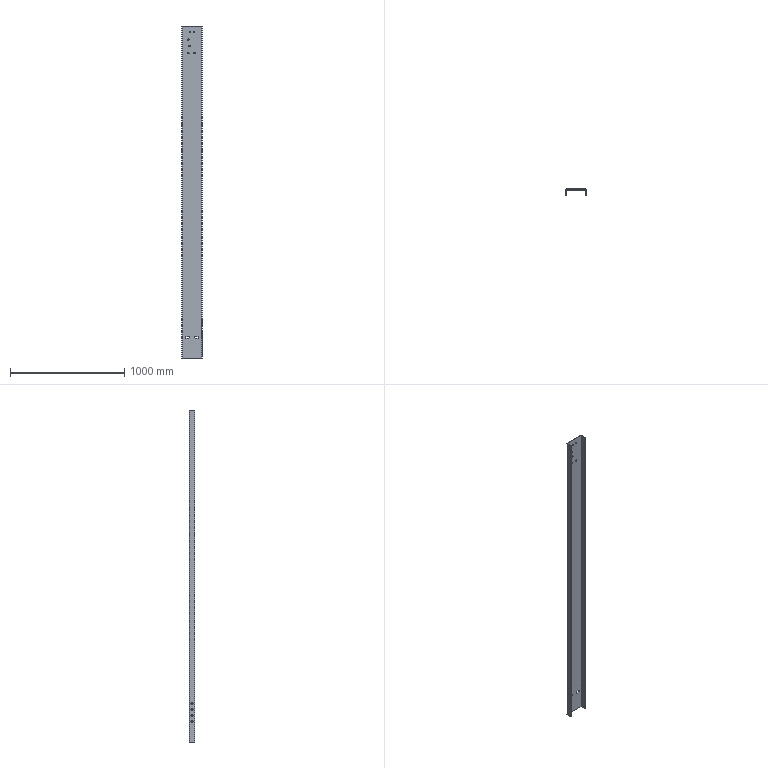Part | SolidWorks | features ICE 3, Fillet 2, FlatPattern 1, SMBaseFlange 1, SheetMetal 1 | 1 solid | 84 faces | box 180 x 50 x 2908 mm | volume 3865801 mm3 | cylinder 46 | plane 38 | commonest cylinder face diameters 13 x32 12 x6 14 x6 2 x2